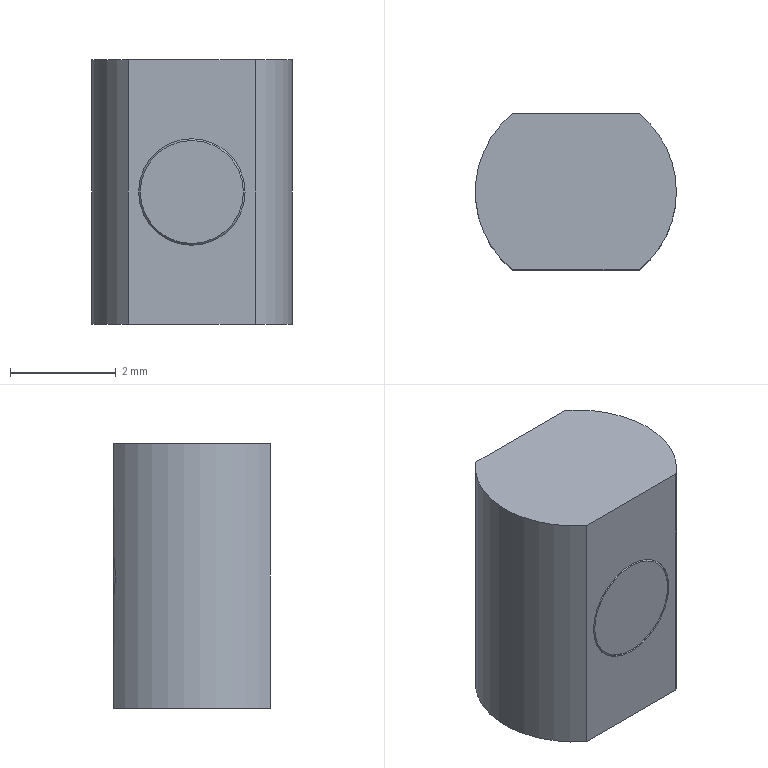Part | SolidWorks | features BaseBody 1 | 1 solid | 32 faces | box 3.8 x 2.95 x 5 mm | volume 47.517 mm3 | plane 19 | cone 8 | cylinder 5 | commonest cylinder face diameters 3.8 x3 2.013 x2
STEP:
#1=CARTESIAN_POINT('',(1.198,0.,-2.5));
#2=VERTEX_POINT('',#1);
#3=CARTESIAN_POINT('',(1.9,1.475,-2.5));
#4=VERTEX_POINT('',#3);
#5=CARTESIAN_POINT('',(0.,1.475,-2.5));
#6=DIRECTION('',(0.,0.,1.));
#7=DIRECTION('',(1.,0.,0.));
#8=AXIS2_PLACEMENT_3D('',#5,#6,#7);
#9=CIRCLE('',#8,1.9);
#10=EDGE_CURVE('',#2,#4,#9,.T.);
#11=ORIENTED_EDGE('',*,*,#10,.T.);
#12=CARTESIAN_POINT('',(1.9,1.475,2.5));
#13=VERTEX_POINT('',#12);
#14=CARTESIAN_POINT('',(1.9,1.475,2.5));
#15=DIRECTION('',(0.,0.,1.));
#16=VECTOR('',#15,1000.);
#17=LINE('',#14,#16);
#18=EDGE_CURVE('',#4,#13,#17,.T.);
#19=ORIENTED_EDGE('',*,*,#18,.T.);
#20=CARTESIAN_POINT('',(1.198,0.,2.5));
#21=VERTEX_POINT('',#20);
#22=CARTESIAN_POINT('',(0.,1.475,2.5));
#23=DIRECTION('',(0.,0.,-1.));
#24=DIRECTION('',(1.,0.,0.));
#25=AXIS2_PLACEMENT_3D('',#22,#23,#24);
#26=CIRCLE('',#25,1.9);
#27=EDGE_CURVE('',#13,#21,#26,.T.);
#28=ORIENTED_EDGE('',*,*,#27,.T.);
#29=CARTESIAN_POINT('',(1.198,0.,2.5));
#30=DIRECTION('',(0.,0.,-1.));
#31=VECTOR('',#30,1000.);
#32=LINE('',#29,#31);
#33=EDGE_CURVE('',#21,#2,#32,.T.);
#34=ORIENTED_EDGE('',*,*,#33,.T.);
#35=EDGE_LOOP('',(#11,#19,#28,#34));
#36=FACE_OUTER_BOUND('',#35,.T.);
#37=CARTESIAN_POINT('',(0.,1.475,2.5));
#38=DIRECTION('',(0.,0.,1.));
#39=DIRECTION('',(1.,0.,0.));
#40=AXIS2_PLACEMENT_3D('',#37,#38,#39);
#41=CYLINDRICAL_SURFACE('',#40,1.9);
#42=ADVANCED_FACE('',(#36),#41,.T.);
#43=CARTESIAN_POINT('',(0.,2.8,-1.1));
#44=VERTEX_POINT('',#43);
#45=CARTESIAN_POINT('',(0.,2.8,1.1));
#46=VERTEX_POINT('',#45);
#47=CARTESIAN_POINT('',(0.,2.8,0.));
#48=DIRECTION('',(0.,1.,0.));
#49=DIRECTION('',(0.,0.,1.));
#50=AXIS2_PLACEMENT_3D('',#47,#48,#49);
#51=CIRCLE('',#50,1.1);
#52=EDGE_CURVE('',#44,#46,#51,.T.);
#53=ORIENTED_EDGE('',*,*,#52,.F.);
#54=CARTESIAN_POINT('',(0.,2.95,-1.25));
#55=VERTEX_POINT('',#54);
#56=CARTESIAN_POINT('',(0.,2.95,-1.25));
#57=DIRECTION('',(0.,0.7071,-0.7071));
#58=VECTOR('',#57,1000.);
#59=LINE('',#56,#58);
#60=EDGE_CURVE('',#44,#55,#59,.T.);
#61=ORIENTED_EDGE('',*,*,#60,.T.);
#62=CARTESIAN_POINT('',(-1.198,2.95,-0.3579));
#63=VERTEX_POINT('',#62);
#64=CARTESIAN_POINT('',(0.,2.95,0.));
#65=DIRECTION('',(0.,1.,0.));
#66=DIRECTION('',(0.,0.,1.));
#67=AXIS2_PLACEMENT_3D('',#64,#65,#66);
#68=CIRCLE('',#67,1.25);
#69=EDGE_CURVE('',#55,#63,#68,.T.);
#70=ORIENTED_EDGE('',*,*,#69,.T.);
#71=CARTESIAN_POINT('',(-1.198,2.95,0.3579));
#72=VERTEX_POINT('',#71);
#73=CARTESIAN_POINT('',(-1.198,2.95,0.3579));
#74=CARTESIAN_POINT('',(-1.236,2.919,0.1208));
#75=CARTESIAN_POINT('',(-1.236,2.919,-0.1208));
#76=CARTESIAN_POINT('',(-1.198,2.95,-0.3579));
#77=B_SPLINE_CURVE_WITH_KNOTS('',3,(#73,#74,#75,#76),.UNSPECIFIED.,.F.,.F.,(4,4),(0.,0.0007164),.UNSPECIFIED.);
#78=EDGE_CURVE('',#72,#63,#77,.T.);
#79=ORIENTED_EDGE('',*,*,#78,.F.);
#80=CARTESIAN_POINT('',(0.,2.95,1.25));
#81=VERTEX_POINT('',#80);
#82=CARTESIAN_POINT('',(0.,2.95,0.));
#83=DIRECTION('',(0.,1.,0.));
#84=DIRECTION('',(0.,0.,1.));
#85=AXIS2_PLACEMENT_3D('',#82,#83,#84);
#86=CIRCLE('',#85,1.25);
#87=EDGE_CURVE('',#72,#81,#86,.T.);
#88=ORIENTED_EDGE('',*,*,#87,.T.);
#89=CARTESIAN_POINT('',(0.,2.95,1.25));
#90=DIRECTION('',(0.,0.7071,0.7071));
#91=VECTOR('',#90,1000.);
#92=LINE('',#89,#91);
#93=EDGE_CURVE('',#46,#81,#92,.T.);
#94=ORIENTED_EDGE('',*,*,#93,.F.);
#95=EDGE_LOOP('',(#53,#61,#70,#79,#88,#94));
#96=FACE_OUTER_BOUND('',#95,.T.);
#97=CARTESIAN_POINT('',(0.,2.95,0.));
#98=DIRECTION('',(0.,1.,0.));
#99=DIRECTION('',(0.,0.,1.));
#100=AXIS2_PLACEMENT_3D('',#97,#98,#99);
#101=CONICAL_SURFACE('',#100,1.25,0.7854);
#102=ADVANCED_FACE('',(#96),#101,.F.);
#103=CARTESIAN_POINT('',(0.,0.,1.006));
#104=VERTEX_POINT('',#103);
#105=CARTESIAN_POINT('',(0.,0.,-1.006));
#106=VERTEX_POINT('',#105);
#107=CARTESIAN_POINT('',(0.,0.,0.));
#108=DIRECTION('',(0.,-1.,0.));
#109=DIRECTION('',(0.,0.,1.));
#110=AXIS2_PLACEMENT_3D('',#107,#108,#109);
#111=CIRCLE('',#110,1.006);
#112=EDGE_CURVE('',#104,#106,#111,.T.);
#113=ORIENTED_EDGE('',*,*,#112,.T.);
#114=CARTESIAN_POINT('',(0.,0.0325,-1.006));
#115=VERTEX_POINT('',#114);
#116=CARTESIAN_POINT('',(0.,0.,-1.006));
#117=DIRECTION('',(0.,1.,0.));
#118=VECTOR('',#117,1000.);
#119=LINE('',#116,#118);
#120=EDGE_CURVE('',#106,#115,#119,.T.);
#121=ORIENTED_EDGE('',*,*,#120,.T.);
#122=CARTESIAN_POINT('',(0.,0.0325,1.006));
#123=VERTEX_POINT('',#122);
#124=CARTESIAN_POINT('',(0.,0.0325,0.));
#125=DIRECTION('',(0.,-1.,0.));
#126=DIRECTION('',(0.,0.,1.));
#127=AXIS2_PLACEMENT_3D('',#124,#125,#126);
#128=CIRCLE('',#127,1.006);
#129=EDGE_CURVE('',#123,#115,#128,.T.);
#130=ORIENTED_EDGE('',*,*,#129,.F.);
#131=CARTESIAN_POINT('',(0.,0.,1.006));
#132=DIRECTION('',(0.,1.,0.));
#133=VECTOR('',#132,1000.);
#134=LINE('',#131,#133);
#135=EDGE_CURVE('',#104,#123,#134,.T.);
#136=ORIENTED_EDGE('',*,*,#135,.F.);
#137=EDGE_LOOP('',(#113,#121,#130,#136));
#138=FACE_OUTER_BOUND('',#137,.T.);
#139=CARTESIAN_POINT('',(0.,0.,0.));
#140=DIRECTION('',(0.,1.,0.));
#141=DIRECTION('',(0.,0.,1.));
#142=AXIS2_PLACEMENT_3D('',#139,#140,#141);
#143=CYLINDRICAL_SURFACE('',#142,1.006);
#144=ADVANCED_FACE('',(#138),#143,.F.);
#145=CARTESIAN_POINT('',(0.,2.95,-0.95));
#146=VERTEX_POINT('',#145);
#147=CARTESIAN_POINT('',(0.,2.95,0.95));
#148=VERTEX_POINT('',#147);
#149=CARTESIAN_POINT('',(0.,2.95,0.));
#150=DIRECTION('',(0.,-1.,0.));
#151=DIRECTION('',(0.,0.,-1.));
#152=AXIS2_PLACEMENT_3D('',#149,#150,#151);
#153=CIRCLE('',#152,0.95);
#154=EDGE_CURVE('',#146,#148,#153,.T.);
#155=ORIENTED_EDGE('',*,*,#154,.T.);
#156=CARTESIAN_POINT('',(0.,2.8,1.1));
#157=DIRECTION('',(0.,-0.7071,0.7071));
#158=VECTOR('',#157,1000.);
#159=LINE('',#156,#158);
#160=EDGE_CURVE('',#148,#46,#159,.T.);
#161=ORIENTED_EDGE('',*,*,#160,.T.);
#162=CARTESIAN_POINT('',(0.,2.8,0.));
#163=DIRECTION('',(0.,1.,0.));
#164=DIRECTION('',(0.,0.,1.));
#165=AXIS2_PLACEMENT_3D('',#162,#163,#164);
#166=CIRCLE('',#165,1.1);
#167=EDGE_CURVE('',#46,#44,#166,.T.);
#168=ORIENTED_EDGE('',*,*,#167,.T.);
#169=CARTESIAN_POINT('',(0.,2.8,-1.1));
#170=DIRECTION('',(0.,-0.7071,-0.7071));
#171=VECTOR('',#170,1000.);
#172=LINE('',#169,#171);
#173=EDGE_CURVE('',#146,#44,#172,.T.);
#174=ORIENTED_EDGE('',*,*,#173,.F.);
#175=EDGE_LOOP('',(#155,#161,#168,#174));
#176=FACE_OUTER_BOUND('',#175,.T.);
#177=CARTESIAN_POINT('',(0.,2.8,0.));
#178=DIRECTION('',(0.,-1.,0.));
#179=DIRECTION('',(0.,0.,-1.));
#180=AXIS2_PLACEMENT_3D('',#177,#178,#179);
#181=CONICAL_SURFACE('',#180,1.1,0.7854);
#182=ADVANCED_FACE('',(#176),#181,.T.);
#183=CARTESIAN_POINT('',(0.,0.,0.974));
#184=VERTEX_POINT('',#183);
#185=CARTESIAN_POINT('',(0.,0.,-0.974));
#186=VERTEX_POINT('',#185);
#187=CARTESIAN_POINT('',(0.,0.,0.));
#188=DIRECTION('',(0.,1.,0.));
#189=DIRECTION('',(0.,0.,1.));
#190=AXIS2_PLACEMENT_3D('',#187,#188,#189);
#191=CIRCLE('',#190,0.974);
#192=EDGE_CURVE('',#184,#186,#191,.T.);
#193=ORIENTED_EDGE('',*,*,#192,.T.);
#194=CARTESIAN_POINT('',(0.,0.0325,-1.006));
#195=DIRECTION('',(0.,0.7071,-0.7071));
#196=VECTOR('',#195,1000.);
#197=LINE('',#194,#196);
#198=EDGE_CURVE('',#186,#115,#197,.T.);
#199=ORIENTED_EDGE('',*,*,#198,.T.);
#200=CARTESIAN_POINT('',(0.,0.0325,0.));
#201=DIRECTION('',(0.,-1.,0.));
#202=DIRECTION('',(0.,0.,1.));
#203=AXIS2_PLACEMENT_3D('',#200,#201,#202);
#204=CIRCLE('',#203,1.006);
#205=EDGE_CURVE('',#115,#123,#204,.T.);
#206=ORIENTED_EDGE('',*,*,#205,.T.);
#207=CARTESIAN_POINT('',(0.,0.0325,1.006));
#208=DIRECTION('',(0.,0.7071,0.7071));
#209=VECTOR('',#208,1000.);
#210=LINE('',#207,#209);
#211=EDGE_CURVE('',#184,#123,#210,.T.);
#212=ORIENTED_EDGE('',*,*,#211,.F.);
#213=EDGE_LOOP('',(#193,#199,#206,#212));
#214=FACE_OUTER_BOUND('',#213,.T.);
#215=CARTESIAN_POINT('',(0.,0.0325,0.));
#216=DIRECTION('',(0.,1.,0.));
#217=DIRECTION('',(0.,0.,1.));
#218=AXIS2_PLACEMENT_3D('',#215,#216,#217);
#219=CONICAL_SURFACE('',#218,1.006,0.7854);
#220=ADVANCED_FACE('',(#214),#219,.T.);
#221=CARTESIAN_POINT('',(0.,1.259,0.));
#222=VERTEX_POINT('',#221);
#223=CARTESIAN_POINT('',(-0.65,1.65,0.));
#224=VERTEX_POINT('',#223);
#225=CARTESIAN_POINT('',(-0.65,1.65,0.));
#226=DIRECTION('',(-0.8572,0.515,0.));
#227=VECTOR('',#226,1000.);
#228=LINE('',#225,#227);
#229=EDGE_CURVE('',#222,#224,#228,.T.);
#230=ORIENTED_EDGE('',*,*,#229,.F.);
#231=CARTESIAN_POINT('',(0.65,1.65,0.));
#232=VERTEX_POINT('',#231);
#233=CARTESIAN_POINT('',(0.65,1.65,0.));
#234=DIRECTION('',(0.8572,0.515,0.));
#235=VECTOR('',#234,1000.);
#236=LINE('',#233,#235);
#237=EDGE_CURVE('',#222,#232,#236,.T.);
#238=ORIENTED_EDGE('',*,*,#237,.T.);
#239=CARTESIAN_POINT('',(0.325,1.65,-0.5629));
#240=VERTEX_POINT('',#239);
#241=CARTESIAN_POINT('',(0.,1.65,0.));
#242=DIRECTION('',(0.,-1.,0.));
#243=DIRECTION('',(-1.,0.,0.));
#244=AXIS2_PLACEMENT_3D('',#241,#242,#243);
#245=CIRCLE('',#244,0.65);
#246=EDGE_CURVE('',#240,#232,#245,.T.);
#247=ORIENTED_EDGE('',*,*,#246,.F.);
#248=CARTESIAN_POINT('',(-0.325,1.65,-0.5629));
#249=VERTEX_POINT('',#248);
#250=CARTESIAN_POINT('',(0.,1.65,0.));
#251=DIRECTION('',(0.,-1.,0.));
#252=DIRECTION('',(-1.,0.,0.));
#253=AXIS2_PLACEMENT_3D('',#250,#251,#252);
#254=CIRCLE('',#253,0.65);
#255=EDGE_CURVE('',#249,#240,#254,.T.);
#256=ORIENTED_EDGE('',*,*,#255,.F.);
#257=CARTESIAN_POINT('',(0.,1.65,0.));
#258=DIRECTION('',(0.,-1.,0.));
#259=DIRECTION('',(-1.,0.,0.));
#260=AXIS2_PLACEMENT_3D('',#257,#258,#259);
#261=CIRCLE('',#260,0.65);
#262=EDGE_CURVE('',#224,#249,#261,.T.);
#263=ORIENTED_EDGE('',*,*,#262,.F.);
#264=EDGE_LOOP('',(#230,#238,#247,#256,#263));
#265=FACE_OUTER_BOUND('',#264,.T.);
#266=CARTESIAN_POINT('',(0.,1.65,0.));
#267=DIRECTION('',(0.,1.,0.));
#268=DIRECTION('',(-1.,0.,0.));
#269=AXIS2_PLACEMENT_3D('',#266,#267,#268);
#270=CONICAL_SURFACE('',#269,0.65,1.03);
#271=ADVANCED_FACE('',(#265),#270,.F.);
#272=ORIENTED_EDGE('',*,*,#18,.F.);
#273=CARTESIAN_POINT('',(1.198,2.95,-2.5));
#274=VERTEX_POINT('',#273);
#275=CARTESIAN_POINT('',(0.,1.475,-2.5));
#276=DIRECTION('',(0.,0.,1.));
#277=DIRECTION('',(1.,0.,0.));
#278=AXIS2_PLACEMENT_3D('',#275,#276,#277);
#279=CIRCLE('',#278,1.9);
#280=EDGE_CURVE('',#4,#274,#279,.T.);
#281=ORIENTED_EDGE('',*,*,#280,.T.);
#282=CARTESIAN_POINT('',(1.198,2.95,-0.3579));
#283=VERTEX_POINT('',#282);
#284=CARTESIAN_POINT('',(1.198,2.95,2.5));
#285=DIRECTION('',(0.,0.,1.));
#286=VECTOR('',#285,1000.);
#287=LINE('',#284,#286);
#288=EDGE_CURVE('',#274,#283,#287,.T.);
#289=ORIENTED_EDGE('',*,*,#288,.T.);
#290=CARTESIAN_POINT('',(1.198,2.95,0.3579));
#291=VERTEX_POINT('',#290);
#292=CARTESIAN_POINT('',(1.198,2.95,-0.3579));
#293=CARTESIAN_POINT('',(1.236,2.919,-0.1208));
#294=CARTESIAN_POINT('',(1.236,2.919,0.1208));
#295=CARTESIAN_POINT('',(1.198,2.95,0.3579));
#296=B_SPLINE_CURVE_WITH_KNOTS('',3,(#292,#293,#294,#295),.UNSPECIFIED.,.F.,.F.,(4,4),(0.,0.0007164),.UNSPECIFIED.);
#297=EDGE_CURVE('',#283,#291,#296,.T.);
#298=ORIENTED_EDGE('',*,*,#297,.T.);
#299=CARTESIAN_POINT('',(1.198,2.95,2.5));
#300=VERTEX_POINT('',#299);
#301=CARTESIAN_POINT('',(1.198,2.95,2.5));
#302=DIRECTION('',(0.,0.,1.));
#303=VECTOR('',#302,1000.);
#304=LINE('',#301,#303);
#305=EDGE_CURVE('',#291,#300,#304,.T.);
#306=ORIENTED_EDGE('',*,*,#305,.T.);
#307=CARTESIAN_POINT('',(0.,1.475,2.5));
#308=DIRECTION('',(0.,0.,-1.));
#309=DIRECTION('',(1.,0.,0.));
#310=AXIS2_PLACEMENT_3D('',#307,#308,#309);
#311=CIRCLE('',#310,1.9);
#312=EDGE_CURVE('',#300,#13,#311,.T.);
#313=ORIENTED_EDGE('',*,*,#312,.T.);
#314=EDGE_LOOP('',(#272,#281,#289,#298,#306,#313));
#315=FACE_OUTER_BOUND('',#314,.T.);
#316=CARTESIAN_POINT('',(0.,1.475,2.5));
#317=DIRECTION('',(0.,0.,1.));
#318=DIRECTION('',(1.,0.,0.));
#319=AXIS2_PLACEMENT_3D('',#316,#317,#318);
#320=CYLINDRICAL_SURFACE('',#319,1.9);
#321=ADVANCED_FACE('',(#315),#320,.T.);
#322=ORIENTED_EDGE('',*,*,#288,.F.);
#323=CARTESIAN_POINT('',(-1.198,2.95,-2.5));
#324=VERTEX_POINT('',#323);
#325=CARTESIAN_POINT('',(1.198,2.95,-2.5));
#326=DIRECTION('',(1.,0.,0.));
#327=VECTOR('',#326,1000.);
#328=LINE('',#325,#327);
#329=EDGE_CURVE('',#324,#274,#328,.T.);
#330=ORIENTED_EDGE('',*,*,#329,.F.);
#331=CARTESIAN_POINT('',(-1.198,2.95,2.5));
#332=DIRECTION('',(0.,0.,-1.));
#333=VECTOR('',#332,1000.);
#334=LINE('',#331,#333);
#335=EDGE_CURVE('',#63,#324,#334,.T.);
#336=ORIENTED_EDGE('',*,*,#335,.F.);
#337=ORIENTED_EDGE('',*,*,#69,.F.);
#338=CARTESIAN_POINT('',(0.,2.95,0.));
#339=DIRECTION('',(0.,1.,0.));
#340=DIRECTION('',(0.,0.,1.));
#341=AXIS2_PLACEMENT_3D('',#338,#339,#340);
#342=CIRCLE('',#341,1.25);
#343=EDGE_CURVE('',#283,#55,#342,.T.);
#344=ORIENTED_EDGE('',*,*,#343,.F.);
#345=EDGE_LOOP('',(#322,#330,#336,#337,#344));
#346=FACE_OUTER_BOUND('',#345,.T.);
#347=CARTESIAN_POINT('',(1.198,2.95,2.5));
#348=DIRECTION('',(0.,-1.,0.));
#349=DIRECTION('',(0.,0.,-1.));
#350=AXIS2_PLACEMENT_3D('',#347,#348,#349);
#351=PLANE('',#350);
#352=ADVANCED_FACE('',(#346),#351,.F.);
#353=ORIENTED_EDGE('',*,*,#10,.F.);
#354=CARTESIAN_POINT('',(-1.198,0.,-2.5));
#355=VERTEX_POINT('',#354);
#356=CARTESIAN_POINT('',(0.,0.,-2.5));
#357=DIRECTION('',(1.,0.,0.));
#358=VECTOR('',#357,1000.);
#359=LINE('',#356,#358);
#360=EDGE_CURVE('',#355,#2,#359,.T.);
#361=ORIENTED_EDGE('',*,*,#360,.F.);
#362=CARTESIAN_POINT('',(0.,1.475,-2.5));
#363=DIRECTION('',(0.,0.,1.));
#364=DIRECTION('',(1.,0.,0.));
#365=AXIS2_PLACEMENT_3D('',#362,#363,#364);
#366=CIRCLE('',#365,1.9);
#367=EDGE_CURVE('',#324,#355,#366,.T.);
#368=ORIENTED_EDGE('',*,*,#367,.F.);
#369=ORIENTED_EDGE('',*,*,#329,.T.);
#370=ORIENTED_EDGE('',*,*,#280,.F.);
#371=EDGE_LOOP('',(#353,#361,#368,#369,#370));
#372=FACE_OUTER_BOUND('',#371,.T.);
#373=CARTESIAN_POINT('',(0.,1.475,-2.5));
#374=DIRECTION('',(0.,0.,1.));
#375=DIRECTION('',(1.,0.,0.));
#376=AXIS2_PLACEMENT_3D('',#373,#374,#375);
#377=PLANE('',#376);
#378=ADVANCED_FACE('',(#372),#377,.F.);
#379=ORIENTED_EDGE('',*,*,#33,.F.);
#380=CARTESIAN_POINT('',(-1.198,0.,2.5));
#381=VERTEX_POINT('',#380);
#382=CARTESIAN_POINT('',(-1.198,0.,2.5));
#383=DIRECTION('',(1.,0.,0.));
#384=VECTOR('',#383,1000.);
#385=LINE('',#382,#384);
#386=EDGE_CURVE('',#381,#21,#385,.T.);
#387=ORIENTED_EDGE('',*,*,#386,.F.);
#388=CARTESIAN_POINT('',(-1.198,0.,2.5));
#389=DIRECTION('',(0.,0.,1.));
#390=VECTOR('',#389,1000.);
#391=LINE('',#388,#390);
#392=EDGE_CURVE('',#355,#381,#391,.T.);
#393=ORIENTED_EDGE('',*,*,#392,.F.);
#394=ORIENTED_EDGE('',*,*,#360,.T.);
#395=EDGE_LOOP('',(#379,#387,#393,#394));
#396=FACE_OUTER_BOUND('',#395,.T.);
#397=ORIENTED_EDGE('',*,*,#112,.F.);
#398=CARTESIAN_POINT('',(0.,0.,0.));
#399=DIRECTION('',(0.,-1.,0.));
#400=DIRECTION('',(0.,0.,1.));
#401=AXIS2_PLACEMENT_3D('',#398,#399,#400);
#402=CIRCLE('',#401,1.006);
#403=EDGE_CURVE('',#106,#104,#402,.T.);
#404=ORIENTED_EDGE('',*,*,#403,.F.);
#405=EDGE_LOOP('',(#397,#404));
#406=FACE_BOUND('',#405,.T.);
#407=CARTESIAN_POINT('',(-1.198,0.,2.5));
#408=DIRECTION('',(0.,1.,0.));
#409=DIRECTION('',(0.,0.,1.));
#410=AXIS2_PLACEMENT_3D('',#407,#408,#409);
#411=PLANE('',#410);
#412=ADVANCED_FACE('',(#396,#406),#411,.F.);
#413=ORIENTED_EDGE('',*,*,#386,.T.);
#414=ORIENTED_EDGE('',*,*,#27,.F.);
#415=ORIENTED_EDGE('',*,*,#312,.F.);
#416=CARTESIAN_POINT('',(-1.198,2.95,2.5));
#417=VERTEX_POINT('',#416);
#418=CARTESIAN_POINT('',(0.,2.95,2.5));
#419=DIRECTION('',(-1.,0.,0.));
#420=VECTOR('',#419,1000.);
#421=LINE('',#418,#420);
#422=EDGE_CURVE('',#300,#417,#421,.T.);
#423=ORIENTED_EDGE('',*,*,#422,.T.);
#424=CARTESIAN_POINT('',(0.,1.475,2.5));
#425=DIRECTION('',(0.,0.,1.));
#426=DIRECTION('',(1.,0.,0.));
#427=AXIS2_PLACEMENT_3D('',#424,#425,#426);
#428=CIRCLE('',#427,1.9);
#429=EDGE_CURVE('',#417,#381,#428,.T.);
#430=ORIENTED_EDGE('',*,*,#429,.T.);
#431=EDGE_LOOP('',(#413,#414,#415,#423,#430));
#432=FACE_OUTER_BOUND('',#431,.T.);
#433=CARTESIAN_POINT('',(0.,1.475,2.5));
#434=DIRECTION('',(0.,0.,1.));
#435=DIRECTION('',(1.,0.,0.));
#436=AXIS2_PLACEMENT_3D('',#433,#434,#435);
#437=PLANE('',#436);
#438=ADVANCED_FACE('',(#432),#437,.T.);
#439=CARTESIAN_POINT('',(-1.198,2.95,2.5));
#440=DIRECTION('',(0.,0.,-1.));
#441=VECTOR('',#440,1000.);
#442=LINE('',#439,#441);
#443=EDGE_CURVE('',#417,#72,#442,.T.);
#444=ORIENTED_EDGE('',*,*,#443,.F.);
#445=ORIENTED_EDGE('',*,*,#422,.F.);
#446=ORIENTED_EDGE('',*,*,#305,.F.);
#447=CARTESIAN_POINT('',(0.,2.95,0.));
#448=DIRECTION('',(0.,1.,0.));
#449=DIRECTION('',(0.,0.,1.));
#450=AXIS2_PLACEMENT_3D('',#447,#448,#449);
#451=CIRCLE('',#450,1.25);
#452=EDGE_CURVE('',#81,#291,#451,.T.);
#453=ORIENTED_EDGE('',*,*,#452,.F.);
#454=ORIENTED_EDGE('',*,*,#87,.F.);
#455=EDGE_LOOP('',(#444,#445,#446,#453,#454));
#456=FACE_OUTER_BOUND('',#455,.T.);
#457=CARTESIAN_POINT('',(1.198,2.95,2.5));
#458=DIRECTION('',(0.,-1.,0.));
#459=DIRECTION('',(0.,0.,-1.));
#460=AXIS2_PLACEMENT_3D('',#457,#458,#459);
#461=PLANE('',#460);
#462=ADVANCED_FACE('',(#456),#461,.F.);
#463=ORIENTED_EDGE('',*,*,#60,.F.);
#464=ORIENTED_EDGE('',*,*,#167,.F.);
#465=ORIENTED_EDGE('',*,*,#93,.T.);
#466=ORIENTED_EDGE('',*,*,#452,.T.);
#467=ORIENTED_EDGE('',*,*,#297,.F.);
#468=ORIENTED_EDGE('',*,*,#343,.T.);
#469=EDGE_LOOP('',(#463,#464,#465,#466,#467,#468));
#470=FACE_OUTER_BOUND('',#469,.T.);
#471=CARTESIAN_POINT('',(0.,2.95,0.));
#472=DIRECTION('',(0.,1.,0.));
#473=DIRECTION('',(0.,0.,1.));
#474=AXIS2_PLACEMENT_3D('',#471,#472,#473);
#475=CONICAL_SURFACE('',#474,1.25,0.7854);
#476=ADVANCED_FACE('',(#470),#475,.F.);
#477=ORIENTED_EDGE('',*,*,#429,.F.);
#478=ORIENTED_EDGE('',*,*,#443,.T.);
#479=ORIENTED_EDGE('',*,*,#78,.T.);
#480=ORIENTED_EDGE('',*,*,#335,.T.);
#481=ORIENTED_EDGE('',*,*,#367,.T.);
#482=ORIENTED_EDGE('',*,*,#392,.T.);
#483=EDGE_LOOP('',(#477,#478,#479,#480,#481,#482));
#484=FACE_OUTER_BOUND('',#483,.T.);
#485=CARTESIAN_POINT('',(0.,1.475,2.5));
#486=DIRECTION('',(0.,0.,1.));
#487=DIRECTION('',(1.,0.,0.));
#488=AXIS2_PLACEMENT_3D('',#485,#486,#487);
#489=CYLINDRICAL_SURFACE('',#488,1.9);
#490=ADVANCED_FACE('',(#484),#489,.T.);
#491=ORIENTED_EDGE('',*,*,#120,.F.);
#492=ORIENTED_EDGE('',*,*,#403,.T.);
#493=ORIENTED_EDGE('',*,*,#135,.T.);
#494=ORIENTED_EDGE('',*,*,#205,.F.);
#495=EDGE_LOOP('',(#491,#492,#493,#494));
#496=FACE_OUTER_BOUND('',#495,.T.);
#497=CARTESIAN_POINT('',(0.,0.,0.));
#498=DIRECTION('',(0.,1.,0.));
#499=DIRECTION('',(0.,0.,1.));
#500=AXIS2_PLACEMENT_3D('',#497,#498,#499);
#501=CYLINDRICAL_SURFACE('',#500,1.006);
#502=ADVANCED_FACE('',(#496),#501,.F.);
#503=ORIENTED_EDGE('',*,*,#160,.F.);
#504=CARTESIAN_POINT('',(0.,2.95,0.));
#505=DIRECTION('',(0.,-1.,0.));
#506=DIRECTION('',(0.,0.,-1.));
#507=AXIS2_PLACEMENT_3D('',#504,#505,#506);
#508=CIRCLE('',#507,0.95);
#509=EDGE_CURVE('',#148,#146,#508,.T.);
#510=ORIENTED_EDGE('',*,*,#509,.T.);
#511=ORIENTED_EDGE('',*,*,#173,.T.);
#512=ORIENTED_EDGE('',*,*,#52,.T.);
#513=EDGE_LOOP('',(#503,#510,#511,#512));
#514=FACE_OUTER_BOUND('',#513,.T.);
#515=CARTESIAN_POINT('',(0.,2.8,0.));
#516=DIRECTION('',(0.,-1.,0.));
#517=DIRECTION('',(0.,0.,-1.));
#518=AXIS2_PLACEMENT_3D('',#515,#516,#517);
#519=CONICAL_SURFACE('',#518,1.1,0.7854);
#520=ADVANCED_FACE('',(#514),#519,.T.);
#521=ORIENTED_EDGE('',*,*,#198,.F.);
#522=CARTESIAN_POINT('',(0.,0.,0.));
#523=DIRECTION('',(0.,1.,0.));
#524=DIRECTION('',(0.,0.,1.));
#525=AXIS2_PLACEMENT_3D('',#522,#523,#524);
#526=CIRCLE('',#525,0.974);
#527=EDGE_CURVE('',#186,#184,#526,.T.);
#528=ORIENTED_EDGE('',*,*,#527,.T.);
#529=ORIENTED_EDGE('',*,*,#211,.T.);
#530=ORIENTED_EDGE('',*,*,#129,.T.);
#531=EDGE_LOOP('',(#521,#528,#529,#530));
#532=FACE_OUTER_BOUND('',#531,.T.);
#533=CARTESIAN_POINT('',(0.,0.0325,0.));
#534=DIRECTION('',(0.,1.,0.));
#535=DIRECTION('',(0.,0.,1.));
#536=AXIS2_PLACEMENT_3D('',#533,#534,#535);
#537=CONICAL_SURFACE('',#536,1.006,0.7854);
#538=ADVANCED_FACE('',(#532),#537,.T.);
#539=CARTESIAN_POINT('',(0.,2.95,0.7506));
#540=VERTEX_POINT('',#539);
#541=CARTESIAN_POINT('',(0.65,2.95,0.3753));
#542=VERTEX_POINT('',#541);
#543=CARTESIAN_POINT('',(0.,2.95,0.7506));
#544=DIRECTION('',(0.866,0.,-0.5));
#545=VECTOR('',#544,1000.);
#546=LINE('',#543,#545);
#547=EDGE_CURVE('',#540,#542,#546,.T.);
#548=ORIENTED_EDGE('',*,*,#547,.F.);
#549=CARTESIAN_POINT('',(-0.65,2.95,0.3753));
#550=VERTEX_POINT('',#549);
#551=CARTESIAN_POINT('',(-0.65,2.95,0.3753));
#552=DIRECTION('',(0.866,0.,0.5));
#553=VECTOR('',#552,1000.);
#554=LINE('',#551,#553);
#555=EDGE_CURVE('',#550,#540,#554,.T.);
#556=ORIENTED_EDGE('',*,*,#555,.F.);
#557=CARTESIAN_POINT('',(-0.65,2.95,-0.3753));
#558=VERTEX_POINT('',#557);
#559=CARTESIAN_POINT('',(-0.65,2.95,0.));
#560=DIRECTION('',(0.,0.,1.));
#561=VECTOR('',#560,1000.);
#562=LINE('',#559,#561);
#563=EDGE_CURVE('',#558,#550,#562,.T.);
#564=ORIENTED_EDGE('',*,*,#563,.F.);
#565=CARTESIAN_POINT('',(0.,2.95,-0.7506));
#566=VERTEX_POINT('',#565);
#567=CARTESIAN_POINT('',(0.,2.95,-0.7506));
#568=DIRECTION('',(-0.866,0.,0.5));
#569=VECTOR('',#568,1000.);
#570=LINE('',#567,#569);
#571=EDGE_CURVE('',#566,#558,#570,.T.);
#572=ORIENTED_EDGE('',*,*,#571,.F.);
#573=CARTESIAN_POINT('',(0.65,2.95,-0.3753));
#574=VERTEX_POINT('',#573);
#575=CARTESIAN_POINT('',(0.65,2.95,-0.3753));
#576=DIRECTION('',(-0.866,0.,-0.5));
#577=VECTOR('',#576,1000.);
#578=LINE('',#575,#577);
#579=EDGE_CURVE('',#574,#566,#578,.T.);
#580=ORIENTED_EDGE('',*,*,#579,.F.);
#581=CARTESIAN_POINT('',(0.65,2.95,0.));
#582=DIRECTION('',(0.,0.,-1.));
#583=VECTOR('',#582,1000.);
#584=LINE('',#581,#583);
#585=EDGE_CURVE('',#542,#574,#584,.T.);
#586=ORIENTED_EDGE('',*,*,#585,.F.);
#587=EDGE_LOOP('',(#548,#556,#564,#572,#580,#586));
#588=FACE_BOUND('',#587,.T.);
#589=ORIENTED_EDGE('',*,*,#154,.F.);
#590=ORIENTED_EDGE('',*,*,#509,.F.);
#591=EDGE_LOOP('',(#589,#590));
#592=FACE_OUTER_BOUND('',#591,.T.);
#593=CARTESIAN_POINT('',(0.65,2.95,0.));
#594=DIRECTION('',(0.,-1.,0.));
#595=DIRECTION('',(0.,0.,-1.));
#596=AXIS2_PLACEMENT_3D('',#593,#594,#595);
#597=PLANE('',#596);
#598=ADVANCED_FACE('',(#588,#592),#597,.F.);
#599=ORIENTED_EDGE('',*,*,#192,.F.);
#600=ORIENTED_EDGE('',*,*,#527,.F.);
#601=EDGE_LOOP('',(#599,#600));
#602=FACE_OUTER_BOUND('',#601,.T.);
#603=CARTESIAN_POINT('',(0.974,0.,0.));
#604=DIRECTION('',(0.,1.,0.));
#605=DIRECTION('',(0.,0.,1.));
#606=AXIS2_PLACEMENT_3D('',#603,#604,#605);
#607=PLANE('',#606);
#608=ADVANCED_FACE('',(#602),#607,.F.);
#609=CARTESIAN_POINT('',(0.65,1.65,0.3753));
#610=VERTEX_POINT('',#609);
#611=CARTESIAN_POINT('',(0.65,1.65,0.3753));
#612=DIRECTION('',(0.,-1.,0.));
#613=VECTOR('',#612,1000.);
#614=LINE('',#611,#613);
#615=EDGE_CURVE('',#542,#610,#614,.T.);
#616=ORIENTED_EDGE('',*,*,#615,.F.);
#617=ORIENTED_EDGE('',*,*,#585,.T.);
#618=CARTESIAN_POINT('',(0.65,1.65,-0.3753));
#619=VERTEX_POINT('',#618);
#620=CARTESIAN_POINT('',(0.65,1.65,-0.3753));
#621=DIRECTION('',(0.,1.,0.));
#622=VECTOR('',#621,1000.);
#623=LINE('',#620,#622);
#624=EDGE_CURVE('',#619,#574,#623,.T.);
#625=ORIENTED_EDGE('',*,*,#624,.F.);
#626=CARTESIAN_POINT('',(0.65,1.65,0.3753));
#627=DIRECTION('',(0.,0.,-1.));
#628=VECTOR('',#627,1000.);
#629=LINE('',#626,#628);
#630=EDGE_CURVE('',#232,#619,#629,.T.);
#631=ORIENTED_EDGE('',*,*,#630,.F.);
#632=CARTESIAN_POINT('',(0.65,1.65,0.3753));
#633=DIRECTION('',(0.,0.,-1.));
#634=VECTOR('',#633,1000.);
#635=LINE('',#632,#634);
#636=EDGE_CURVE('',#610,#232,#635,.T.);
#637=ORIENTED_EDGE('',*,*,#636,.F.);
#638=EDGE_LOOP('',(#616,#617,#625,#631,#637));
#639=FACE_OUTER_BOUND('',#638,.T.);
#640=CARTESIAN_POINT('',(0.65,1.65,0.3753));
#641=DIRECTION('',(1.,0.,0.));
#642=DIRECTION('',(0.,0.,-1.));
#643=AXIS2_PLACEMENT_3D('',#640,#641,#642);
#644=PLANE('',#643);
#645=ADVANCED_FACE('',(#639),#644,.F.);
#646=CARTESIAN_POINT('',(0.,1.65,0.7506));
#647=VERTEX_POINT('',#646);
#648=CARTESIAN_POINT('',(0.,1.65,0.7506));
#649=DIRECTION('',(0.,-1.,0.));
#650=VECTOR('',#649,1000.);
#651=LINE('',#648,#650);
#652=EDGE_CURVE('',#540,#647,#651,.T.);
#653=ORIENTED_EDGE('',*,*,#652,.F.);
#654=ORIENTED_EDGE('',*,*,#547,.T.);
#655=ORIENTED_EDGE('',*,*,#615,.T.);
#656=CARTESIAN_POINT('',(0.325,1.65,0.5629));
#657=VERTEX_POINT('',#656);
#658=CARTESIAN_POINT('',(0.,1.65,0.7506));
#659=DIRECTION('',(0.866,0.,-0.5));
#660=VECTOR('',#659,1000.);
#661=LINE('',#658,#660);
#662=EDGE_CURVE('',#657,#610,#661,.T.);
#663=ORIENTED_EDGE('',*,*,#662,.F.);
#664=CARTESIAN_POINT('',(0.,1.65,0.7506));
#665=DIRECTION('',(0.866,0.,-0.5));
#666=VECTOR('',#665,1000.);
#667=LINE('',#664,#666);
#668=EDGE_CURVE('',#647,#657,#667,.T.);
#669=ORIENTED_EDGE('',*,*,#668,.F.);
#670=EDGE_LOOP('',(#653,#654,#655,#663,#669));
#671=FACE_OUTER_BOUND('',#670,.T.);
#672=CARTESIAN_POINT('',(0.,1.65,0.7506));
#673=DIRECTION('',(0.5,0.,0.866));
#674=DIRECTION('',(0.866,0.,-0.5));
#675=AXIS2_PLACEMENT_3D('',#672,#673,#674);
#676=PLANE('',#675);
#677=ADVANCED_FACE('',(#671),#676,.F.);
#678=CARTESIAN_POINT('',(-0.65,1.65,0.3753));
#679=VERTEX_POINT('',#678);
#680=CARTESIAN_POINT('',(-0.65,1.65,0.3753));
#681=DIRECTION('',(0.,-1.,0.));
#682=VECTOR('',#681,1000.);
#683=LINE('',#680,#682);
#684=EDGE_CURVE('',#550,#679,#683,.T.);
#685=ORIENTED_EDGE('',*,*,#684,.F.);
#686=ORIENTED_EDGE('',*,*,#555,.T.);
#687=ORIENTED_EDGE('',*,*,#652,.T.);
#688=CARTESIAN_POINT('',(-0.325,1.65,0.5629));
#689=VERTEX_POINT('',#688);
#690=CARTESIAN_POINT('',(-0.65,1.65,0.3753));
#691=DIRECTION('',(0.866,0.,0.5));
#692=VECTOR('',#691,1000.);
#693=LINE('',#690,#692);
#694=EDGE_CURVE('',#689,#647,#693,.T.);
#695=ORIENTED_EDGE('',*,*,#694,.F.);
#696=CARTESIAN_POINT('',(-0.65,1.65,0.3753));
#697=DIRECTION('',(0.866,0.,0.5));
#698=VECTOR('',#697,1000.);
#699=LINE('',#696,#698);
#700=EDGE_CURVE('',#679,#689,#699,.T.);
#701=ORIENTED_EDGE('',*,*,#700,.F.);
#702=EDGE_LOOP('',(#685,#686,#687,#695,#701));
#703=FACE_OUTER_BOUND('',#702,.T.);
#704=CARTESIAN_POINT('',(-0.65,1.65,0.3753));
#705=DIRECTION('',(-0.5,0.,0.866));
#706=DIRECTION('',(0.866,0.,0.5));
#707=AXIS2_PLACEMENT_3D('',#704,#705,#706);
#708=PLANE('',#707);
#709=ADVANCED_FACE('',(#703),#708,.F.);
#710=CARTESIAN_POINT('',(-0.65,1.65,-0.3753));
#711=VERTEX_POINT('',#710);
#712=CARTESIAN_POINT('',(-0.65,1.65,-0.3753));
#713=DIRECTION('',(0.,-1.,0.));
#714=VECTOR('',#713,1000.);
#715=LINE('',#712,#714);
#716=EDGE_CURVE('',#558,#711,#715,.T.);
#717=ORIENTED_EDGE('',*,*,#716,.F.);
#718=ORIENTED_EDGE('',*,*,#563,.T.);
#719=ORIENTED_EDGE('',*,*,#684,.T.);
#720=CARTESIAN_POINT('',(-0.65,1.65,-0.3753));
#721=DIRECTION('',(0.,0.,1.));
#722=VECTOR('',#721,1000.);
#723=LINE('',#720,#722);
#724=EDGE_CURVE('',#224,#679,#723,.T.);
#725=ORIENTED_EDGE('',*,*,#724,.F.);
#726=CARTESIAN_POINT('',(-0.65,1.65,-0.3753));
#727=DIRECTION('',(0.,0.,1.));
#728=VECTOR('',#727,1000.);
#729=LINE('',#726,#728);
#730=EDGE_CURVE('',#711,#224,#729,.T.);
#731=ORIENTED_EDGE('',*,*,#730,.F.);
#732=EDGE_LOOP('',(#717,#718,#719,#725,#731));
#733=FACE_OUTER_BOUND('',#732,.T.);
#734=CARTESIAN_POINT('',(-0.65,1.65,-0.3753));
#735=DIRECTION('',(-1.,0.,0.));
#736=DIRECTION('',(0.,0.,1.));
#737=AXIS2_PLACEMENT_3D('',#734,#735,#736);
#738=PLANE('',#737);
#739=ADVANCED_FACE('',(#733),#738,.F.);
#740=CARTESIAN_POINT('',(0.,1.65,-0.7506));
#741=VERTEX_POINT('',#740);
#742=CARTESIAN_POINT('',(0.,1.65,-0.7506));
#743=DIRECTION('',(0.,-1.,0.));
#744=VECTOR('',#743,1000.);
#745=LINE('',#742,#744);
#746=EDGE_CURVE('',#566,#741,#745,.T.);
#747=ORIENTED_EDGE('',*,*,#746,.F.);
#748=ORIENTED_EDGE('',*,*,#571,.T.);
#749=ORIENTED_EDGE('',*,*,#716,.T.);
#750=CARTESIAN_POINT('',(0.,1.65,-0.7506));
#751=DIRECTION('',(-0.866,0.,0.5));
#752=VECTOR('',#751,1000.);
#753=LINE('',#750,#752);
#754=EDGE_CURVE('',#249,#711,#753,.T.);
#755=ORIENTED_EDGE('',*,*,#754,.F.);
#756=CARTESIAN_POINT('',(0.,1.65,-0.7506));
#757=DIRECTION('',(-0.866,0.,0.5));
#758=VECTOR('',#757,1000.);
#759=LINE('',#756,#758);
#760=EDGE_CURVE('',#741,#249,#759,.T.);
#761=ORIENTED_EDGE('',*,*,#760,.F.);
#762=EDGE_LOOP('',(#747,#748,#749,#755,#761));
#763=FACE_OUTER_BOUND('',#762,.T.);
#764=CARTESIAN_POINT('',(0.,1.65,-0.7506));
#765=DIRECTION('',(-0.5,0.,-0.866));
#766=DIRECTION('',(-0.866,0.,0.5));
#767=AXIS2_PLACEMENT_3D('',#764,#765,#766);
#768=PLANE('',#767);
#769=ADVANCED_FACE('',(#763),#768,.F.);
#770=ORIENTED_EDGE('',*,*,#624,.T.);
#771=ORIENTED_EDGE('',*,*,#579,.T.);
#772=ORIENTED_EDGE('',*,*,#746,.T.);
#773=CARTESIAN_POINT('',(0.65,1.65,-0.3753));
#774=DIRECTION('',(-0.866,0.,-0.5));
#775=VECTOR('',#774,1000.);
#776=LINE('',#773,#775);
#777=EDGE_CURVE('',#240,#741,#776,.T.);
#778=ORIENTED_EDGE('',*,*,#777,.F.);
#779=CARTESIAN_POINT('',(0.65,1.65,-0.3753));
#780=DIRECTION('',(-0.866,0.,-0.5));
#781=VECTOR('',#780,1000.);
#782=LINE('',#779,#781);
#783=EDGE_CURVE('',#619,#240,#782,.T.);
#784=ORIENTED_EDGE('',*,*,#783,.F.);
#785=EDGE_LOOP('',(#770,#771,#772,#778,#784));
#786=FACE_OUTER_BOUND('',#785,.T.);
#787=CARTESIAN_POINT('',(0.65,1.65,-0.3753));
#788=DIRECTION('',(0.5,0.,-0.866));
#789=DIRECTION('',(-0.866,0.,-0.5));
#790=AXIS2_PLACEMENT_3D('',#787,#788,#789);
#791=PLANE('',#790);
#792=ADVANCED_FACE('',(#786),#791,.F.);
#793=ORIENTED_EDGE('',*,*,#662,.T.);
#794=ORIENTED_EDGE('',*,*,#636,.T.);
#795=CARTESIAN_POINT('',(0.,1.65,0.));
#796=DIRECTION('',(0.,-1.,0.));
#797=DIRECTION('',(-1.,0.,0.));
#798=AXIS2_PLACEMENT_3D('',#795,#796,#797);
#799=CIRCLE('',#798,0.65);
#800=EDGE_CURVE('',#232,#657,#799,.T.);
#801=ORIENTED_EDGE('',*,*,#800,.T.);
#802=EDGE_LOOP('',(#793,#794,#801));
#803=FACE_OUTER_BOUND('',#802,.T.);
#804=CARTESIAN_POINT('',(0.,1.65,0.));
#805=DIRECTION('',(0.,1.,0.));
#806=DIRECTION('',(0.,0.,1.));
#807=AXIS2_PLACEMENT_3D('',#804,#805,#806);
#808=PLANE('',#807);
#809=ADVANCED_FACE('',(#803),#808,.T.);
#810=ORIENTED_EDGE('',*,*,#630,.T.);
#811=ORIENTED_EDGE('',*,*,#783,.T.);
#812=ORIENTED_EDGE('',*,*,#246,.T.);
#813=EDGE_LOOP('',(#810,#811,#812));
#814=FACE_OUTER_BOUND('',#813,.T.);
#815=CARTESIAN_POINT('',(0.,1.65,0.));
#816=DIRECTION('',(0.,1.,0.));
#817=DIRECTION('',(0.,0.,1.));
#818=AXIS2_PLACEMENT_3D('',#815,#816,#817);
#819=PLANE('',#818);
#820=ADVANCED_FACE('',(#814),#819,.T.);
#821=ORIENTED_EDGE('',*,*,#694,.T.);
#822=ORIENTED_EDGE('',*,*,#668,.T.);
#823=CARTESIAN_POINT('',(0.,1.65,0.));
#824=DIRECTION('',(0.,-1.,0.));
#825=DIRECTION('',(-1.,0.,0.));
#826=AXIS2_PLACEMENT_3D('',#823,#824,#825);
#827=CIRCLE('',#826,0.65);
#828=EDGE_CURVE('',#657,#689,#827,.T.);
#829=ORIENTED_EDGE('',*,*,#828,.T.);
#830=EDGE_LOOP('',(#821,#822,#829));
#831=FACE_OUTER_BOUND('',#830,.T.);
#832=CARTESIAN_POINT('',(0.,1.65,0.));
#833=DIRECTION('',(0.,1.,0.));
#834=DIRECTION('',(0.,0.,1.));
#835=AXIS2_PLACEMENT_3D('',#832,#833,#834);
#836=PLANE('',#835);
#837=ADVANCED_FACE('',(#831),#836,.T.);
#838=ORIENTED_EDGE('',*,*,#724,.T.);
#839=ORIENTED_EDGE('',*,*,#700,.T.);
#840=CARTESIAN_POINT('',(0.,1.65,0.));
#841=DIRECTION('',(0.,-1.,0.));
#842=DIRECTION('',(-1.,0.,0.));
#843=AXIS2_PLACEMENT_3D('',#840,#841,#842);
#844=CIRCLE('',#843,0.65);
#845=EDGE_CURVE('',#689,#224,#844,.T.);
#846=ORIENTED_EDGE('',*,*,#845,.T.);
#847=EDGE_LOOP('',(#838,#839,#846));
#848=FACE_OUTER_BOUND('',#847,.T.);
#849=CARTESIAN_POINT('',(0.,1.65,0.));
#850=DIRECTION('',(0.,1.,0.));
#851=DIRECTION('',(0.,0.,1.));
#852=AXIS2_PLACEMENT_3D('',#849,#850,#851);
#853=PLANE('',#852);
#854=ADVANCED_FACE('',(#848),#853,.T.);
#855=ORIENTED_EDGE('',*,*,#754,.T.);
#856=ORIENTED_EDGE('',*,*,#730,.T.);
#857=ORIENTED_EDGE('',*,*,#262,.T.);
#858=EDGE_LOOP('',(#855,#856,#857));
#859=FACE_OUTER_BOUND('',#858,.T.);
#860=CARTESIAN_POINT('',(0.,1.65,0.));
#861=DIRECTION('',(0.,1.,0.));
#862=DIRECTION('',(0.,0.,1.));
#863=AXIS2_PLACEMENT_3D('',#860,#861,#862);
#864=PLANE('',#863);
#865=ADVANCED_FACE('',(#859),#864,.T.);
#866=ORIENTED_EDGE('',*,*,#777,.T.);
#867=ORIENTED_EDGE('',*,*,#760,.T.);
#868=ORIENTED_EDGE('',*,*,#255,.T.);
#869=EDGE_LOOP('',(#866,#867,#868));
#870=FACE_OUTER_BOUND('',#869,.T.);
#871=CARTESIAN_POINT('',(0.,1.65,0.));
#872=DIRECTION('',(0.,1.,0.));
#873=DIRECTION('',(0.,0.,1.));
#874=AXIS2_PLACEMENT_3D('',#871,#872,#873);
#875=PLANE('',#874);
#876=ADVANCED_FACE('',(#870),#875,.T.);
#877=ORIENTED_EDGE('',*,*,#237,.F.);
#878=ORIENTED_EDGE('',*,*,#229,.T.);
#879=ORIENTED_EDGE('',*,*,#845,.F.);
#880=ORIENTED_EDGE('',*,*,#828,.F.);
#881=ORIENTED_EDGE('',*,*,#800,.F.);
#882=EDGE_LOOP('',(#877,#878,#879,#880,#881));
#883=FACE_OUTER_BOUND('',#882,.T.);
#884=CARTESIAN_POINT('',(0.,1.65,0.));
#885=DIRECTION('',(0.,1.,0.));
#886=DIRECTION('',(-1.,0.,0.));
#887=AXIS2_PLACEMENT_3D('',#884,#885,#886);
#888=CONICAL_SURFACE('',#887,0.65,1.03);
#889=ADVANCED_FACE('',(#883),#888,.F.);
#890=CLOSED_SHELL('',(#42,#102,#144,#182,#220,#271,#321,#352,#378,#412,#438,#462,#476,#490,#502,#520,#538,#598,#608,#645,#677,#709,#739,#769,#792,#809,#820,#837,#854,#865,#876,#889));
#891=MANIFOLD_SOLID_BREP('',#890);
#892=CARTESIAN_POINT('',(0.,0.,0.));
#893=DIRECTION('',(0.,0.,1.));
#894=DIRECTION('',(1.,0.,0.));
#895=AXIS2_PLACEMENT_3D('',#892,#893,#894);
#896=(LENGTH_UNIT()NAMED_UNIT(*)SI_UNIT(.MILLI.,.METRE.));
#897=UNCERTAINTY_MEASURE_WITH_UNIT(LENGTH_MEASURE(0.00001),#896,'','');
#898=(NAMED_UNIT(*)PLANE_ANGLE_UNIT()SI_UNIT($,.RADIAN.));
#899=(NAMED_UNIT(*)SI_UNIT($,.STERADIAN.)SOLID_ANGLE_UNIT());
#900=(GEOMETRIC_REPRESENTATION_CONTEXT(3)GLOBAL_UNCERTAINTY_ASSIGNED_CONTEXT((#897))GLOBAL_UNIT_ASSIGNED_CONTEXT((#896,#898,#899))REPRESENTATION_CONTEXT('',''));
#901=ADVANCED_BREP_SHAPE_REPRESENTATION('',(#891,#895),#900);